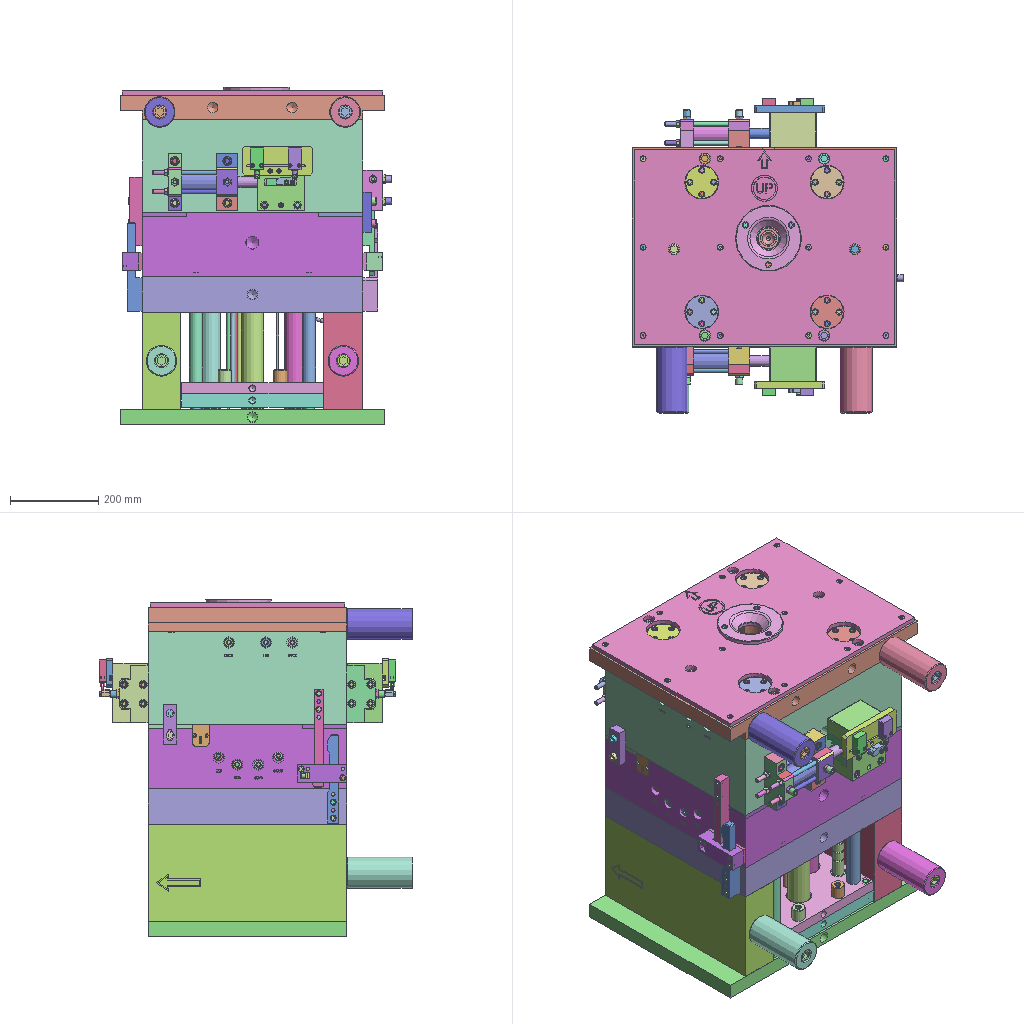Assembly | STEP file | 162 different items | 424 placed | box 616 x 711 x 765 mm
Parts list (item | name | quantity | parent item | size | volume):
1 | AA | x1 | in 12HPB013-WZP-GM-4.17_objects | 500 x 450 x 210 mm | 28750729 mm3
2 | AD | x1 | in 12HPB013-WZP-GM-4.17_objects | 600 x 450 x 55 mm | 12937855 mm3
3 | BB | x1 | in 12HPB013-WZP-GM-4.17_objects | 500 x 450 x 145 mm | 21236141 mm3
4 | BD | x1 | in 12HPB013-WZP-GM-4.17_objects | 600 x 450 x 35 mm | 8925184 mm3
5 | BDB | x1 | in 12HPB013-WZP-GM-4.17_objects | 500 x 450 x 80 mm | 15672052 mm3
6 | CC01 | x1 | in 12HPB013-WZP-GM-4.17_objects | 88 x 450 x 220 mm | 8457298 mm3
7 | CC02 | x1 | in 12HPB013-WZP-GM-4.17_objects | 88 x 450 x 220 mm | 8509495 mm3
8 | DZDB | x1 | in 12HPB013-WZP-GM-4.17_objects | 320 x 450 x 30 mm | 3701626 mm3
9 | DZMB | x1 | in 12HPB013-WZP-GM-4.17_objects | 320 x 450 x 25 mm | 2980315 mm3
10 | LJD | x6 | in 12HPB013-WZP-GM-4.17_objects | 12 x 12 x 15 mm | 521.973 mm3
11 | M10.00-20 | x2 | in 12HPB013-WZP-GM-4.17_objects | 560 x 368 x 18 mm | 10650 mm3
12 | M10.00-30.00 | x4 | in 12HPB013-WZP-GM-4.17_objects | 16 x 16 x 40 mm | 4032 mm3
13 | M10.00-45 | x2 | in 12HPB013-WZP-GM-4.17_objects | 46 x 86 x 70 mm | 11598 mm3
14 | M10.00-85 | x8 | in 12HPB013-WZP-GM-4.17_objects | 16 x 16 x 171.5 mm | 14936 mm3
15 | M10.00-90.00 | x3 | in 12HPB013-WZP-GM-4.17_objects | 16 x 16 x 100 mm | 8744 mm3
16 | M12.00-50.00 | x6 | in 12HPB013-WZP-GM-4.17_objects | 18 x 18 x 62 mm | 8110 mm3
17 | M12.00-55.00 | x4 | in 12HPB013-WZP-GM-4.17_objects | 18 x 18 x 67 mm | 8675 mm3
18 | M12.00-95.00 | x6 | in 12HPB013-WZP-GM-4.17_objects | 18 x 18 x 107 mm | 13199 mm3
19 | M16.00-45.00 | x6 | in 12HPB013-WZP-GM-4.17_objects | 24 x 24 x 72.5 mm | 17180 mm3
20 | M20.00-160.00 | x4 | in 12HPB013-WZP-GM-4.17_objects | 30 x 180 x 30 mm | 61632 mm3
21 | M4.00-15 | x4 | in 12HPB013-WZP-GM-4.17_objects | 27 x 670 x 7 mm | 844.151 mm3
22 | M6.00-20.00 | x1 | in 12HPB013-WZP-GM-4.17_objects | 10 x 10 x 26 mm | 965.752 mm3
23 | M8.00-15.00 | x16 | in 12HPB013-WZP-GM-4.17_objects | 13 x 13 x 23 mm | 1644 mm3
24 | M8.00-35 | x3 | in 12HPB013-WZP-GM-4.17_objects | 33.038 x 270 x 682.52 mm | 5048 mm3
25 | M8.00-50.00 | x7 | in 12HPB013-WZP-GM-4.17_objects | 13 x 13 x 83 mm | 4660 mm3
26 | PTM6.00-15.00 | x4 | in 12HPB013-WZP-GM-4.17_objects | 12 x 12 x 16.55 mm | 586.414 mm3
27 | PTM6.00-20.00 | x12 | in 12HPB013-WZP-GM-4.17_objects | 12 x 12 x 16.55 mm | 586.414 mm3
28 | PTM8.00-20 | x4 | in 12HPB013-WZP-GM-4.17_objects | 97.883 x 291 x 103.532 mm | 3365 mm3
29 | solid 1 | x2 | in 12HPB013-WZP-GM-4.17_objects | 10 x 15 x 10 mm | 148.735 mm3
30 | solid 100 | x6 | in 12HPB013-WZP-GM-4.17_objects | 10 x 10 x 21 mm | 824.381 mm3
31 | solid 101 | x6 | in 12HPB013-WZP-GM-4.17_objects | 10 x 10 x 31 mm | 1107 mm3
32 | solid 102 | x3 | in 12HPB013-WZP-GM-4.17_objects | 50 x 30 x 22 mm | 22296 mm3
33 | solid 103 | x3 | in 12HPB013-WZP-GM-4.17_objects | 50 x 30 x 24.5 mm | 26652 mm3
34 | solid 104 | x1 | in 12HPB013-WZP-GM-4.17_objects | 10 x 10 x 137.677 mm | 10813 mm3
35 | solid 105 | x1 | in 12HPB013-WZP-GM-4.17_objects | 10 x 10 x 127.677 mm | 10028 mm3
36 | solid 106 | x1 | in 12HPB013-WZP-GM-4.17_objects | 22 x 22 x 89.177 mm | 33899 mm3
37 | solid 107 | x4 | in 12HPB013-WZP-GM-4.17_objects | 70 x 150 x 70 mm | 514377 mm3
38 | solid 108 | x1 | in 12HPB013-WZP-GM-4.17_objects | 136.142 x 176.757 x 187.43 mm | 2148805 mm3
39 | solid 109 | x2 | in 12HPB013-WZP-GM-4.17_objects | 22 x 22 x 134.177 mm | 51005 mm3
40 | solid 110 | x1 | in 12HPB013-WZP-GM-4.17_objects | 187 x 12 x 12 mm | 21149 mm3
41 | solid 111 | x1 | in 12HPB013-WZP-GM-4.17_objects | 182 x 12 x 12 mm | 20584 mm3
42 | solid 112 | x1 | in 12HPB013-WZP-GM-4.17_objects | 25 x 25 x 12 mm | 5890 mm3
43 | solid 113 | x1 | in 12HPB013-WZP-GM-4.17_objects | 43.011 x 46.317 x 12 mm | 8861 mm3
44 | solid 114 | x1 | in 12HPB013-WZP-GM-4.17_objects | 45.902 x 37.289 x 12 mm | 8376 mm3
45 | solid 115 | x1 | in 12HPB013-WZP-GM-4.17_objects | 63.638 x 19 x 149.358 mm | 31086 mm3
46 | solid 118 | x2 | in 12HPB013-WZP-GM-4.17_objects | 29 x 19.63 x 22.667 mm | 5092 mm3
47 | solid 119 | x2 | in 12HPB013-WZP-GM-4.17_objects | 44.094 x 10 x 106.274 mm | 5918 mm3
48 | solid 120 | x1 | in 12HPB013-WZP-GM-4.17_objects | 10 x 96 x 10 mm | 5250 mm3
49 | solid 121 | x2 | in 12HPB013-WZP-GM-4.17_objects | 29 x 8 x 8 mm | 1458 mm3
50 | solid 123 | x1 | in 12HPB013-WZP-GM-4.17_objects | 80 x 30 x 80 mm | 120680 mm3
51 | solid 124 | x1 | in 12HPB013-WZP-GM-4.17_objects | 80 x 30 x 80 mm | 143867 mm3
52 | solid 125 | x4 | in 12HPB013-WZP-GM-4.17_objects | 55 x 55 x 431 mm | 847132 mm3
53 | solid 126 | x4 | in 12HPB013-WZP-GM-4.17_objects | 76 x 76 x 210 mm | 403335 mm3
54 | solid 127 | x4 | in 12HPB013-WZP-GM-4.17_objects | 70 x 70 x 136 mm | 255628 mm3
55 | solid 128 | x3 | in 12HPB013-WZP-GM-4.17_objects | 100 x 100 x 10 mm | 72323 mm3
56 | solid 129 | x1 | in 12HPB013-WZP-GM-4.17_objects | 27.5 x 25 x 223 mm | 95743 mm3
57 | solid 13 | x1 | in 12HPB013-WZP-GM-4.17_objects | 25 x 38 x 49.5 mm | 43620 mm3
58 | solid 130 | x1 | in 12HPB013-WZP-GM-4.17_objects | 33.5 x 25 x 200.006 mm | 103265 mm3
59 | solid 131 | x2 | in 12HPB013-WZP-GM-4.17_objects | 30 x 100 x 59.496 mm | 142436 mm3
60 | solid 132 | x2 | in 12HPB013-WZP-GM-4.17_objects | 80 x 30 x 59.496 mm | 109836 mm3
61 | solid 134 | x2 | in 12HPB013-WZP-GM-4.17_objects | 29 x 19.63 x 22.667 mm | 5092 mm3
62 | solid 135 | x1 | in 12HPB013-WZP-GM-4.17_objects | 111.404 x 17.72 x 178 mm | 11788 mm3
63 | solid 136 | x1 | in 12HPB013-WZP-GM-4.17_objects | 113.804 x 11.5 x 178 mm | 11895 mm3
64 | solid 137 | x1 | in 12HPB013-WZP-GM-4.17_objects | 85 x 78 x 119.504 mm | 501919 mm3
65 | solid 139 | x1 | in 12HPB013-WZP-GM-4.17_objects | 10 x 144 x 10 mm | 7521 mm3
66 | solid 14 | x2 | in 12HPB013-WZP-GM-4.17_objects | 125 x 30 x 25 mm | 81564 mm3
67 | solid 141 | x4 | in 12HPB013-WZP-GM-4.17_objects | 20 x 20 x 60.51 mm | 11893 mm3
68 | solid 142 | x1 | in 12HPB013-WZP-GM-4.17_objects | 10 x 60 x 10 mm | 4502 mm3
69 | solid 143 | x1 | in 12HPB013-WZP-GM-4.17_objects | 12 x 10 x 70 mm | 6864 mm3
70 | solid 144 | x2 | in 12HPB013-WZP-GM-4.17_objects | 16 x 95 x 16 mm | 8373 mm3
71 | solid 145 | x4 | in 12HPB013-WZP-GM-4.17_objects | 18 x 57 x 18 mm | 7569 mm3
72 | solid 146 | x1 | in 12HPB013-WZP-GM-4.17_objects | 10 x 57 x 10 mm | 4325 mm3
73 | solid 147 | x2 | in 12HPB013-WZP-GM-4.17_objects | 10 x 16 x 10 mm | 680.986 mm3
74 | solid 148 | x1 | in 12HPB013-WZP-GM-4.17_objects | 42 x 45 x 17 mm | 16851 mm3
75 | solid 149 | x2 | in 12HPB013-WZP-GM-4.17_objects | 16 x 82 x 16 mm | 7351 mm3
76 | solid 150 | x2 | in 12HPB013-WZP-GM-4.17_objects | 10 x 20 x 10 mm | 794.444 mm3
77 | solid 151 | x2 | in 12HPB013-WZP-GM-4.17_objects | 10 x 60 x 10 mm | 1925 mm3
78 | solid 152 | x1 | in 12HPB013-WZP-GM-4.17_objects | 105 x 60 x 70 mm | 303902 mm3
79 | solid 153 | x4 | in 12HPB013-WZP-GM-4.17_objects | 35 x 35 x 195 mm | 128650 mm3
80 | solid 155 | x2 | in 12HPB013-WZP-GM-4.17_objects | 20 x 30 x 90 mm | 46899 mm3
81 | solid 158 | x1 | in 12HPB013-WZP-GM-4.17_objects | 187.742 x 202 x 123.694 mm | 1808093 mm3
82 | solid 159 | x1 | in 12HPB013-WZP-GM-4.17_objects | 250 x 290 x 170.5 mm | 8891009 mm3
83 | solid 160 | x1 | in 12HPB013-WZP-GM-4.17_objects | 105 x 60 x 70 mm | 303902 mm3
84 | solid 161 | x1 | in 12HPB013-WZP-GM-4.17_objects | 150 x 150 x 30 mm | 414170 mm3
85 | solid 163 | x4 | in 12HPB013-WZP-GM-4.17_objects | 30 x 16 x 70.3 mm | 23738 mm3
86 | solid 165 | x8 | in 12HPB013-WZP-GM-4.17_objects | 9.238 x 4.7 x 8 mm | 187.183 mm3
87 | solid 167 | x1 | in 12HPB013-WZP-GM-4.17_objects | 160 x 15 x 65 mm | 135897 mm3
88 | solid 168 | x1 | in 12HPB013-WZP-GM-4.17_objects | 105 x 80 x 135 mm | 660934 mm3
89 | solid 169 | x1 | in 12HPB013-WZP-GM-4.17_objects | 87.731 x 140.677 x 218.816 mm | 678741 mm3
90 | solid 17 | x1 | in 12HPB013-WZP-GM-4.17_objects | 13 x 15 x 530.22 mm | 41997 mm3
91 | solid 18 | x4 | in 12HPB013-WZP-GM-4.17_objects | 11 x 11 x 477.132 mm | 11113 mm3
92 | solid 2 | x3 | in 12HPB013-WZP-GM-4.17_objects | 55 x 13 x 13 mm | 3119 mm3
93 | solid 22 | x4 | in 12HPB013-WZP-GM-4.17_objects | 30 x 30 x 270.5 mm | 130641 mm3
94 | solid 23 | x6 | in 12HPB013-WZP-GM-4.17_objects | 18 x 18 x 54 mm | 7284 mm3
95 | solid 24 | x4 | in 12HPB013-WZP-GM-4.17_objects | 35 x 35 x 391 mm | 277592 mm3
96 | solid 25 | x6 | in 12HPB013-WZP-GM-4.17_objects | 24 x 24 x 283.5 mm | 59748 mm3
97 | solid 26 | x4 | in 12HPB013-WZP-GM-4.17_objects | 18 x 18 x 58 mm | 7736 mm3
98 | solid 27 | x4 | in 12HPB013-WZP-GM-4.17_objects | 40 x 40 x 53 mm | 26012 mm3
99 | solid 28 | x1 | in 12HPB013-WZP-GM-4.17_objects | 72.72 x 100 x 55.001 mm | 242059 mm3
100 | solid 29 | x1 | in 12HPB013-WZP-GM-4.17_objects | 66.011 x 30 x 133.284 mm | 68942 mm3
101 | solid 3 | x2 | in 12HPB013-WZP-GM-4.17_objects | 39 x 13 x 13 mm | 2314 mm3
102 | solid 30 | x1 | in 12HPB013-WZP-GM-4.17_objects | 177.202 x 210.598 x 142.71 mm | 224641 mm3
103 | solid 31 | x1 | in 12HPB013-WZP-GM-4.17_objects | 250 x 290 x 72 mm | 2895131 mm3
104 | solid 32 | x1 | in 12HPB013-WZP-GM-4.17_objects | 37 x 83.675 x 87.541 mm | 174258 mm3
105 | solid 33 | x1 | in 12HPB013-WZP-GM-4.17_objects | 30 x 215.791 x 35 mm | 148988 mm3
106 | solid 34 | x1 | in 12HPB013-WZP-GM-4.17_objects | 30 x 202.213 x 35 mm | 142973 mm3
107 | solid 37 | x1 | in 12HPB013-WZP-GM-4.17_objects | 41.968 x 175 x 77.179 mm | 118228 mm3
108 | solid 4 | x2 | in 12HPB013-WZP-GM-4.17_objects | 44.5 x 13 x 13 mm | 2591 mm3
109 | solid 40 | x1 | in 12HPB013-WZP-GM-4.17_objects | 85 x 160 x 10 mm | 124096 mm3
110 | solid 41 | x11 | in 12HPB013-WZP-GM-4.17_objects | 32 x 19.63 x 22.667 mm | 5655 mm3
111 | solid 42 | x1 | in 12HPB013-WZP-GM-4.17_objects | 16 x 16 x 15 mm | 2748 mm3
112 | solid 47 | x2 | in 12HPB013-WZP-GM-4.17_objects | 24 x 20 x 79.442 mm | 29301 mm3
113 | solid 48 | x1 | in 12HPB013-WZP-GM-4.17_objects | 160 x 15 x 65 mm | 135897 mm3
114 | solid 49 | x1 | in 12HPB013-WZP-GM-4.17_objects | 105 x 80 x 135 mm | 660934 mm3
115 | solid 5 | x3 | in 12HPB013-WZP-GM-4.17_objects | 55 x 13 x 13 mm | 3119 mm3
116 | solid 50 | x2 | in 12HPB013-WZP-GM-4.17_objects | 82 x 50 x 50 mm | 57962 mm3
117 | solid 51 | x2 | in 12HPB013-WZP-GM-4.17_objects | 16 x 82 x 16 mm | 7351 mm3
118 | solid 52 | x2 | in 12HPB013-WZP-GM-4.17_objects | 16 x 95 x 16 mm | 8373 mm3
119 | solid 53 | x2 | in 12HPB013-WZP-GM-4.17_objects | 10 x 60 x 10 mm | 1925 mm3
120 | solid 54 | x4 | in 12HPB013-WZP-GM-4.17_objects | 18 x 57 x 18 mm | 7569 mm3
121 | solid 55 | x2 | in 12HPB013-WZP-GM-4.17_objects | 10 x 16 x 10 mm | 680.986 mm3
122 | solid 56 | x1 | in 12HPB013-WZP-GM-4.17_objects | 10 x 60 x 10 mm | 4502 mm3
123 | solid 57 | x1 | in 12HPB013-WZP-GM-4.17_objects | 12 x 10 x 70 mm | 6864 mm3
124 | solid 58 | x2 | in 12HPB013-WZP-GM-4.17_objects | 10 x 20 x 10 mm | 794.444 mm3
125 | solid 59 | x1 | in 12HPB013-WZP-GM-4.17_objects | 42 x 45 x 17 mm | 16851 mm3
126 | solid 6 | x2 | in 12HPB013-WZP-GM-4.17_objects | 39 x 13 x 13 mm | 2314 mm3
127 | solid 60 | x1 | in 12HPB013-WZP-GM-4.17_objects | 10 x 57 x 10 mm | 4325 mm3
128 | solid 63 | x4 | in 12HPB013-WZP-GM-4.17_objects | 15 x 15 x 74.066 mm | 5678 mm3
129 | solid 64 | x4 | in 12HPB013-WZP-GM-4.17_objects | 8 x 8 x 549.996 mm | 8877 mm3
130 | solid 65 | x1 | in 12HPB013-WZP-GM-4.17_objects | 25 x 29.916 x 10 mm | 5820 mm3
131 | solid 67 | x3 | in 12HPB013-WZP-GM-4.17_objects | 20 x 30 x 10 mm | 5338 mm3
132 | solid 68 | x7 | in 12HPB013-WZP-GM-4.17_objects | 15 x 15 x 408.49 mm | 32672 mm3
133 | solid 69 | x2 | in 12HPB013-WZP-GM-4.17_objects | 10 x 10 x 408.49 mm | 11851 mm3
134 | solid 7 | x2 | in 12HPB013-WZP-GM-4.17_objects | 44.5 x 13 x 13 mm | 2591 mm3
135 | solid 70 | x2 | in 12HPB013-WZP-GM-4.17_objects | 15 x 15 x 466.378 mm | 37218 mm3
136 | solid 71 | x1 | in 12HPB013-WZP-GM-4.17_objects | 15 x 15 x 512.106 mm | 40810 mm3
137 | solid 72 | x2 | in 12HPB013-WZP-GM-4.17_objects | 50 x 50 x 220 mm | 430674 mm3
138 | solid 73 | x2 | in 12HPB013-WZP-GM-4.17_objects | 45 x 45 x 220 mm | 348635 mm3
139 | solid 74 | x3 | in 12HPB013-WZP-GM-4.17_objects | 45 x 45 x 220 mm | 348635 mm3
140 | solid 77 | x6 | in 12HPB013-WZP-GM-4.17_objects | 20 x 20 x 5 mm | 1227 mm3
141 | solid 78 | x4 | in 12HPB013-WZP-GM-4.17_objects | 30 x 30 x 30 mm | 18536 mm3
142 | solid 79 | x1 | in 12HPB013-WZP-GM-4.17_objects | 590 x 440 x 10 mm | 2194749 mm3
143 | solid 8 | x2 | in 12HPB013-WZP-GM-4.17_objects | 30 x 100 x 80 mm | 186268 mm3
144 | solid 80 | x4 | in 12HPB013-WZP-GM-4.17_objects | 10 x 10 x 40 mm | 2747 mm3
145 | solid 81 | x2 | in 12HPB013-WZP-GM-4.17_objects | 133 x 12 x 12 mm | 15042 mm3
146 | solid 82 | x2 | in 12HPB013-WZP-GM-4.17_objects | 12 x 12 x 51 mm | 5768 mm3
147 | solid 83 | x9 | in 12HPB013-WZP-GM-4.17_objects | 32 x 19.63 x 22.667 mm | 5655 mm3
148 | solid 85 | x4 | in 12HPB013-WZP-GM-4.17_objects | 55.5 x 8 x 8 mm | 2790 mm3
149 | solid 86 | x2 | in 12HPB013-WZP-GM-4.17_objects | 8 x 112 x 40 mm | 34018 mm3
150 | solid 87 | x1 | in 12HPB013-WZP-GM-4.17_objects | 30.5 x 56 x 14 mm | 14654 mm3
151 | solid 88 | x1 | in 12HPB013-WZP-GM-4.17_objects | 36 x 112 x 40 mm | 94873 mm3
152 | solid 89 | x4 | in 12HPB013-WZP-GM-4.17_objects | 35 x 35 x 20 mm | 17200 mm3
153 | solid 9 | x1 | in 12HPB013-WZP-GM-4.17_objects | 100 x 100 x 10 mm | 72272 mm3
154 | solid 90 | x4 | in 12HPB013-WZP-GM-4.17_objects | 13 x 13 x 33 mm | 2177 mm3
155 | solid 91 | x4 | in 12HPB013-WZP-GM-4.17_objects | 33 x 33 x 159 mm | 75495 mm3
156 | solid 92 | x4 | in 12HPB013-WZP-GM-4.17_objects | 39.5 x 8 x 8 mm | 1985 mm3
157 | solid 93 | x1 | in 12HPB013-WZP-GM-4.17_objects | 36 x 112 x 40 mm | 94873 mm3
158 | solid 94 | x4 | in 12HPB013-WZP-GM-4.17_objects | 45 x 8 x 8 mm | 2262 mm3
159 | solid 95 | x1 | in 12HPB013-WZP-GM-4.17_objects | 30.5 x 56 x 14 mm | 14654 mm3
160 | solid 96 | x1 | in 12HPB013-WZP-GM-4.17_objects | 33.5 x 25 x 199.996 mm | 103324 mm3
161 | solid 97 | x1 | in 12HPB013-WZP-GM-4.17_objects | 27.5 x 25 x 223 mm | 95863 mm3
162 | solid 99 | x4 | in 12HPB013-WZP-GM-4.17_objects | 75 x 75 x 12 mm | 46733 mm3